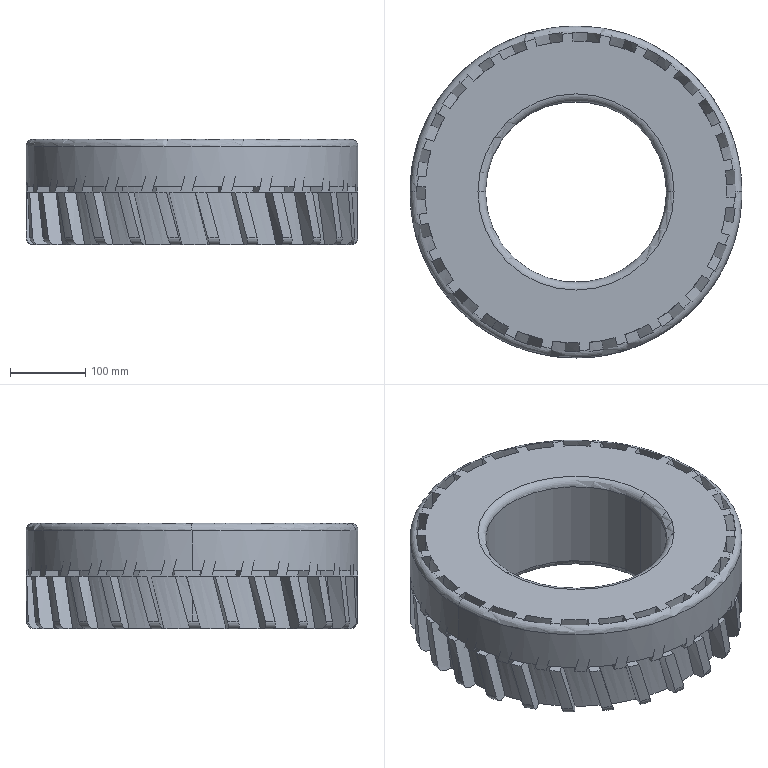Part | SolidWorks | features BlendCut 2, CirPattern 2, Extrusion 1, Fillet 1 | 1 solid | 300 faces | box 440 x 440 x 140 mm | volume 12462431 mm3 | spline 182 | plane 54 | torus 33 | cylinder 31 | commonest cylinder face diameters 440 x29 240 x2